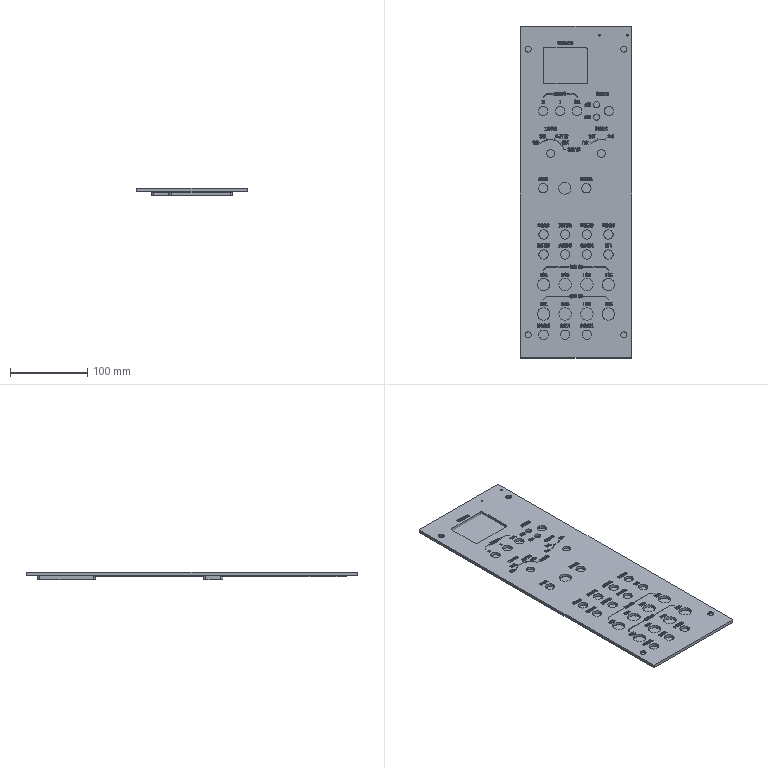NC program | Mastercam | posted with a generic post
Lines 8665 to 9754 of 54676:
(4 FEM |TOOL - 4|DIA. OFF. - 4|LEN. - 4|TOOL DIA. - 4.)
N7506 T4 M6
N7508 G0 G54 G90 X119.431 Y19.1 C0. B0. S7000 M3
N7510 G43 H4 Z50.
N7512 Z-4.248
N7514 G3 X119.931 Y18.6 I.5 F3000.
N7516 G1 X121.958
N7518 X121.975
N7520 G3 X122.265 Y18.641 J1.034
N7522 G1 X122.328 Y18.664
N7524 X122.449 Y18.722
N7526 X122.56 Y18.798
N7528 X122.659 Y18.889
N7530 X122.742 Y18.994
N7532 X122.81 Y19.11
N7534 X122.859 Y19.235
N7536 X122.888 Y19.366
N7538 G3 X122.9 Y19.529 I-1.149 J.163
N7540 G1 X122.899 Y19.539
N7542 X122.9 Y21.623
N7544 Y21.647 Z-4.249
N7546 Y21.71 Z-4.263
N7548 Y21.771 Z-4.303
N7550 Y21.808 Z-4.359
N7552 Y21.82 Z-4.423
N7554 Y21.808 Z-4.488
N7556 Y21.771 Z-4.544
N7558 Y21.71 Z-4.584
N7560 Y21.623 Z-4.599
N7562 Y19.539
N7564 Y19.531
N7566 G2 X122.876 Y19.3 I-1.123
N7568 G1 X122.859 Y19.235
N7570 X122.81 Y19.11
N7572 X122.742 Y18.994
N7574 X122.659 Y18.889
N7576 X122.56 Y18.798
N7578 X122.449 Y18.722
N7580 X122.328 Y18.664
N7582 X122.201 Y18.624
N7584 G2 X121.98 Y18.6 I-.221 J.986
N7586 G1 X121.958
N7588 X119.931
N7590 X119.907 Z-4.6
N7592 X119.845 Z-4.614
N7594 X119.783 Z-4.653
N7596 X119.746 Z-4.71
N7598 X119.734 Z-4.774
N7600 X119.746 Z-4.838
N7602 X119.783 Z-4.894
N7604 X119.845 Z-4.934
N7606 X119.931 Z-4.949
N7608 X121.958
N7610 X121.975
N7612 G3 X122.265 Y18.641 J1.034
N7614 G1 X122.328 Y18.664
N7616 X122.449 Y18.722
N7618 X122.56 Y18.798
N7620 X122.659 Y18.889
N7622 X122.742 Y18.994
N7624 X122.81 Y19.11
N7626 X122.859 Y19.235
N7628 X122.888 Y19.366
N7630 G3 X122.9 Y19.529 I-1.149 J.163
N7632 G1 X122.899 Y19.539
N7634 X122.9 Y21.623
N7636 Y21.647 Z-4.95
N7638 Y21.71 Z-4.964
N7640 Y21.771 Z-5.004
N7642 Y21.808 Z-5.06
N7644 Y21.82 Z-5.124
N7646 Y21.808 Z-5.188
N7648 Y21.771 Z-5.245
N7650 Y21.71 Z-5.284
N7652 Y21.623 Z-5.299
N7654 Y19.539
N7656 Y19.531
N7658 G2 X122.876 Y19.3 I-1.123
N7660 G1 X122.859 Y19.235
N7662 X122.81 Y19.11
N7664 X122.742 Y18.994
N7666 X122.659 Y18.889
N7668 X122.56 Y18.798
N7670 X122.449 Y18.722
N7672 X122.328 Y18.664
N7674 X122.201 Y18.624
N7676 G2 X121.98 Y18.6 I-.221 J.986
N7678 G1 X121.958
N7680 X119.931
N7682 X119.907 Z-5.3
N7684 X119.845 Z-5.314
N7686 X119.783 Z-5.354
N7688 X119.746 Z-5.41
N7690 X119.734 Z-5.474
N7692 X119.746 Z-5.539
N7694 X119.783 Z-5.595
N7696 X119.845 Z-5.635
N7698 X119.931 Z-5.65
N7700 X121.958
N7702 X121.975
N7704 G3 X122.265 Y18.641 J1.034
N7706 G1 X122.328 Y18.664
N7708 X122.449 Y18.722
N7710 X122.56 Y18.798
N7712 X122.659 Y18.889
N7714 X122.742 Y18.994
N7716 X122.81 Y19.11
N7718 X122.859 Y19.235
N7720 X122.888 Y19.366
N7722 G3 X122.9 Y19.529 I-1.149 J.163
N7724 G1 X122.899 Y19.539
N7726 X122.9 Y21.623
N7728 Y21.656 Z-5.652
N7730 Y21.709 Z-5.673
N7732 Y21.744 Z-5.708
N7734 Y21.764 Z-5.775
N7736 Y21.744 Z-5.842
N7738 Y21.709 Z-5.877
N7740 Y21.656 Z-5.897
N7742 Y21.623 Z-5.9
N7744 Y19.539
N7746 Y19.531
N7748 G2 X122.876 Y19.3 I-1.123
N7750 G1 X122.859 Y19.235
N7752 X122.81 Y19.11
N7754 X122.742 Y18.994
N7756 X122.659 Y18.889
N7758 X122.56 Y18.798
N7760 X122.449 Y18.722
N7762 X122.328 Y18.664
N7764 X122.201 Y18.624
N7766 G2 X121.98 Y18.6 I-.221 J.986
N7768 G1 X121.958
N7770 X119.931
N7772 X119.924 Z-5.897
N7774 Z-5.886
N7776 X119.931 Z-5.883
N7778 X121.958
N7780 X121.975
N7782 G3 X122.265 Y18.641 J1.034
N7784 G1 X122.328 Y18.664
N7786 X122.449 Y18.722
N7788 X122.56 Y18.798
N7790 X122.659 Y18.889
N7792 X122.742 Y18.994
N7794 X122.81 Y19.11
N7796 X122.859 Y19.235
N7798 X122.888 Y19.366
N7800 G3 X122.9 Y19.529 I-1.149 J.163
N7802 G1 X122.899 Y19.539
N7804 X122.9 Y21.623
N7806 G3 X122.4 Y22.123 I-.5
N7808 G0 Z50.
N7810 X119.395 Y8.9
N7812 Z-4.248
N7814 G2 X119.895 Y9.4 I.5
N7816 G1 X121.958
N7818 X121.975
N7820 G2 X122.265 Y9.359 J-1.034
N7822 G1 X122.389 Y9.31
N7824 X122.506 Y9.242
N7826 X122.611 Y9.159
N7828 X122.742 Y9.006
N7830 X122.81 Y8.889
N7832 X122.876 Y8.7
N7834 G2 X122.9 Y8.481 I-.981 J-.219
N7836 G1 Y8.46
N7838 Y6.328
N7840 Y6.304 Z-4.249
N7842 Y6.242 Z-4.263
N7844 Y6.18 Z-4.303
N7846 Y6.143 Z-4.359
N7848 Y6.131 Z-4.423
N7850 Y6.143 Z-4.488
N7852 Y6.18 Z-4.544
N7854 Y6.242 Z-4.584
N7856 Y6.328 Z-4.599
N7858 Y8.46
N7860 Y8.468
N7862 G3 X122.876 Y8.7 I-1.134
N7864 G1 X122.859 Y8.765
N7866 X122.81 Y8.889
N7868 X122.742 Y9.006
N7870 X122.611 Y9.159
N7872 X122.506 Y9.242
N7874 X122.389 Y9.31
N7876 X122.201 Y9.376
N7878 G3 X121.98 Y9.4 I-.221 J-.986
N7880 G1 X121.958
N7882 X119.895
N7884 X119.871 Z-4.6
N7886 X119.808 Z-4.614
N7888 X119.747 Z-4.653
N7890 X119.71 Z-4.71
N7892 X119.698 Z-4.774
N7894 X119.71 Z-4.838
N7896 X119.747 Z-4.894
N7898 X119.808 Z-4.934
N7900 X119.895 Z-4.949
N7902 X121.958
N7904 X121.975
N7906 G2 X122.265 Y9.359 J-1.034
N7908 G1 X122.389 Y9.31
N7910 X122.506 Y9.242
N7912 X122.611 Y9.159
N7914 X122.742 Y9.006
N7916 X122.81 Y8.889
N7918 X122.876 Y8.7
N7920 G2 X122.9 Y8.481 I-.981 J-.219
N7922 G1 Y8.46
N7924 Y6.328
N7926 Y6.304 Z-4.95
N7928 Y6.242 Z-4.964
N7930 Y6.18 Z-5.004
N7932 Y6.143 Z-5.06
N7934 Y6.131 Z-5.124
N7936 Y6.143 Z-5.188
N7938 Y6.18 Z-5.245
N7940 Y6.242 Z-5.284
N7942 Y6.328 Z-5.299
N7944 Y8.46
N7946 Y8.468
N7948 G3 X122.876 Y8.7 I-1.134
N7950 G1 X122.859 Y8.765
N7952 X122.81 Y8.889
N7954 X122.742 Y9.006
N7956 X122.611 Y9.159
N7958 X122.506 Y9.242
N7960 X122.389 Y9.31
N7962 X122.201 Y9.376
N7964 G3 X121.98 Y9.4 I-.221 J-.986
N7966 G1 X121.958
N7968 X119.895
N7970 X119.871 Z-5.3
N7972 X119.808 Z-5.314
N7974 X119.747 Z-5.354
N7976 X119.71 Z-5.41
N7978 X119.698 Z-5.474
N7980 X119.71 Z-5.539
N7982 X119.747 Z-5.595
N7984 X119.808 Z-5.635
N7986 X119.895 Z-5.65
N7988 X121.958
N7990 X121.975
N7992 G2 X122.265 Y9.359 J-1.034
N7994 G1 X122.389 Y9.31
N7996 X122.506 Y9.242
N7998 X122.611 Y9.159
N8000 X122.742 Y9.006
N8002 X122.81 Y8.889
N8004 X122.876 Y8.7
N8006 G2 X122.9 Y8.481 I-.981 J-.219
N8008 G1 Y8.46
N8010 Y6.328
N8012 Y6.295 Z-5.652
N8014 Y6.242 Z-5.673
N8016 Y6.207 Z-5.708
N8018 Y6.187 Z-5.775
N8020 Y6.207 Z-5.842
N8022 Y6.242 Z-5.877
N8024 Y6.295 Z-5.897
N8026 Y6.328 Z-5.9
N8028 Y8.46
N8030 Y8.468
N8032 G3 X122.876 Y8.7 I-1.134
N8034 G1 X122.859 Y8.765
N8036 X122.81 Y8.889
N8038 X122.742 Y9.006
N8040 X122.611 Y9.159
N8042 X122.506 Y9.242
N8044 X122.389 Y9.31
N8046 X122.201 Y9.376
N8048 G3 X121.98 Y9.4 I-.221 J-.986
N8050 G1 X121.958
N8052 X119.895
N8054 X119.888 Z-5.897
N8056 Z-5.886
N8058 X119.895 Z-5.884
N8060 X121.958
N8062 X121.975
N8064 G2 X122.265 Y9.359 J-1.034
N8066 G1 X122.389 Y9.31
N8068 X122.506 Y9.242
N8070 X122.611 Y9.159
N8072 X122.742 Y9.006
N8074 X122.81 Y8.889
N8076 X122.876 Y8.7
N8078 G2 X122.9 Y8.481 I-.981 J-.219
N8080 G1 Y8.46
N8082 Y6.328
N8084 G2 X122.4 Y5.828 I-.5
N8086 G0 Z50.
N8088 X90.674 Y8.9
N8090 Z-4.248
N8092 G3 X90.174 Y9.4 I-.5
N8094 G1 X88.04
N8096 X88.032
N8098 G3 X87.8 Y9.376 J-1.133
N8100 G1 X87.735 Y9.359
N8102 X87.61 Y9.31
N8104 X87.494 Y9.242
N8106 X87.389 Y9.159
N8108 X87.298 Y9.06
N8110 X87.222 Y8.949
N8112 X87.164 Y8.828
N8114 X87.124 Y8.7
N8116 G3 X87.1 Y8.481 I.979 J-.219
N8118 G1 Y8.46
N8120 Y6.292
N8122 Y6.268 Z-4.249
N8124 Y6.206 Z-4.263
N8126 Y6.144 Z-4.303
N8128 Y6.107 Z-4.359
N8130 Y6.095 Z-4.423
N8132 Y6.107 Z-4.488
N8134 Y6.144 Z-4.544
N8136 Y6.206 Z-4.584
N8138 Y6.292 Z-4.599
N8140 Y8.46
N8142 Y8.468
N8144 G2 X87.124 Y8.7 I1.135
N8146 G1 X87.141 Y8.765
N8148 X87.19 Y8.89
N8150 X87.258 Y9.006
N8152 X87.341 Y9.111
N8154 X87.44 Y9.202
N8156 X87.551 Y9.278
N8158 X87.672 Y9.336
N8160 X87.8 Y9.376
N8162 G2 X88.019 Y9.4 I.219 J-.978
N8164 G1 X88.04
N8166 X90.174
N8168 X90.198 Z-4.6
N8170 X90.261 Z-4.614
N8172 X90.322 Z-4.653
N8174 X90.359 Z-4.71
N8176 X90.371 Z-4.774
N8178 X90.359 Z-4.838
N8180 X90.322 Z-4.894
N8182 X90.261 Z-4.934
N8184 X90.174 Z-4.949
N8186 X88.04
N8188 X88.032
N8190 G3 X87.8 Y9.376 J-1.133
N8192 G1 X87.735 Y9.359
N8194 X87.61 Y9.31
N8196 X87.494 Y9.242
N8198 X87.389 Y9.159
N8200 X87.298 Y9.06
N8202 X87.222 Y8.949
N8204 X87.164 Y8.828
N8206 X87.124 Y8.7
N8208 G3 X87.1 Y8.481 I.979 J-.219
N8210 G1 Y8.46
N8212 Y6.292
N8214 Y6.268 Z-4.95
N8216 Y6.206 Z-4.964
N8218 Y6.144 Z-5.004
N8220 Y6.107 Z-5.06
N8222 Y6.095 Z-5.124
N8224 Y6.107 Z-5.188
N8226 Y6.144 Z-5.245
N8228 Y6.206 Z-5.284
N8230 Y6.292 Z-5.299
N8232 Y8.46
N8234 Y8.468
N8236 G2 X87.124 Y8.7 I1.135
N8238 G1 X87.141 Y8.765
N8240 X87.19 Y8.89
N8242 X87.258 Y9.006
N8244 X87.341 Y9.111
N8246 X87.44 Y9.202
N8248 X87.551 Y9.278
N8250 X87.672 Y9.336
N8252 X87.8 Y9.376
N8254 G2 X88.019 Y9.4 I.219 J-.978
N8256 G1 X88.04
N8258 X90.174
N8260 X90.198 Z-5.3
N8262 X90.261 Z-5.314
N8264 X90.322 Z-5.354
N8266 X90.359 Z-5.41
N8268 X90.371 Z-5.474
N8270 X90.359 Z-5.539
N8272 X90.322 Z-5.595
N8274 X90.261 Z-5.635
N8276 X90.174 Z-5.65
N8278 X88.04
N8280 X88.032
N8282 G3 X87.8 Y9.376 J-1.133
N8284 G1 X87.735 Y9.359
N8286 X87.61 Y9.31
N8288 X87.494 Y9.242
N8290 X87.389 Y9.159
N8292 X87.298 Y9.06
N8294 X87.222 Y8.949
N8296 X87.164 Y8.828
N8298 X87.124 Y8.7
N8300 G3 X87.1 Y8.481 I.979 J-.219
N8302 G1 Y8.46
N8304 Y6.292
N8306 Y6.259 Z-5.652
N8308 Y6.206 Z-5.673
N8310 Y6.171 Z-5.708
N8312 Y6.151 Z-5.775
N8314 Y6.171 Z-5.842
N8316 Y6.206 Z-5.877
N8318 Y6.259 Z-5.897
N8320 Y6.292 Z-5.9
N8322 Y8.46
N8324 Y8.468
N8326 G2 X87.124 Y8.7 I1.135
N8328 G1 X87.141 Y8.765
N8330 X87.19 Y8.89
N8332 X87.258 Y9.006
N8334 X87.341 Y9.111
N8336 X87.44 Y9.202
N8338 X87.551 Y9.278
N8340 X87.672 Y9.336
N8342 X87.8 Y9.376
N8344 G2 X88.019 Y9.4 I.219 J-.978
N8346 G1 X88.04
N8348 X90.174
N8350 X90.181 Z-5.897
N8352 Z-5.886
N8354 X90.174 Z-5.884
N8356 X88.04
N8358 X88.032
N8360 G3 X87.8 Y9.376 J-1.133
N8362 G1 X87.735 Y9.359
N8364 X87.61 Y9.31
N8366 X87.494 Y9.242
N8368 X87.389 Y9.159
N8370 X87.298 Y9.06
N8372 X87.222 Y8.949
N8374 X87.164 Y8.828
N8376 X87.124 Y8.7
N8378 G3 X87.1 Y8.481 I.979 J-.219
N8380 G1 Y8.46
N8382 Y6.292
N8384 G3 X87.6 Y5.792 I.5
N8386 G0 Z50.
N8388 X90.711 Y19.1
N8390 Z-4.248
N8392 G2 X90.211 Y18.6 I-.5
N8394 G1 X88.04
N8396 X88.025
N8398 G2 X87.735 Y18.641 J1.036
N8400 G1 X87.672 Y18.664
N8402 X87.551 Y18.722
N8404 X87.389 Y18.841
N8406 X87.298 Y18.94
N8408 X87.222 Y19.051
N8410 X87.163 Y19.172
N8412 X87.124 Y19.3
N8414 X87.104 Y19.433
N8416 X87.1 Y21.587
N8418 Y21.611 Z-4.249
N8420 Y21.673 Z-4.263
N8422 Y21.735 Z-4.303
N8424 Y21.772 Z-4.359
N8426 Y21.784 Z-4.423
N8428 Y21.772 Z-4.488
N8430 Y21.735 Z-4.544
N8432 Y21.673 Z-4.584
N8434 Y21.587 Z-4.599
N8436 Y19.539
N8438 Y19.531
N8440 G3 X87.124 Y19.3 I1.123
N8442 G1 X87.141 Y19.235
N8444 X87.191 Y19.11
N8446 X87.258 Y18.994
N8448 X87.341 Y18.889
N8450 X87.439 Y18.798
N8452 X87.551 Y18.722
N8454 X87.672 Y18.664
N8456 X87.735 Y18.641
N8458 X87.865 Y18.612
N8460 G3 X88.031 Y18.6 I.166 J1.164
N8462 G1 X88.04
N8464 X90.211
N8466 X90.234 Z-4.6
N8468 X90.297 Z-4.614
N8470 X90.358 Z-4.653
N8472 X90.395 Z-4.71
N8474 X90.408 Z-4.774
N8476 X90.395 Z-4.838
N8478 X90.358 Z-4.894
N8480 X90.297 Z-4.934
N8482 X90.211 Z-4.949
N8484 X88.04
N8486 X88.025
N8488 G2 X87.735 Y18.641 J1.036
N8490 G1 X87.672 Y18.664
N8492 X87.551 Y18.722
N8494 X87.389 Y18.841
N8496 X87.298 Y18.94
N8498 X87.222 Y19.051
N8500 X87.163 Y19.172
N8502 X87.124 Y19.3
N8504 X87.104 Y19.433
N8506 X87.1 Y21.587
N8508 Y21.611 Z-4.95
N8510 Y21.673 Z-4.964
N8512 Y21.735 Z-5.004
N8514 Y21.772 Z-5.06
N8516 Y21.784 Z-5.124
N8518 Y21.772 Z-5.188
N8520 Y21.735 Z-5.245
N8522 Y21.673 Z-5.284
N8524 Y21.587 Z-5.299
N8526 Y19.539
N8528 Y19.531
N8530 G3 X87.124 Y19.3 I1.123
N8532 G1 X87.141 Y19.235
N8534 X87.191 Y19.11
N8536 X87.258 Y18.994
N8538 X87.341 Y18.889
N8540 X87.439 Y18.798
N8542 X87.551 Y18.722
N8544 X87.672 Y18.664
N8546 X87.735 Y18.641
N8548 X87.865 Y18.612
N8550 G3 X88.031 Y18.6 I.166 J1.164
N8552 G1 X88.04
N8554 X90.211
N8556 X90.234 Z-5.3
N8558 X90.297 Z-5.314
N8560 X90.358 Z-5.354
N8562 X90.395 Z-5.41
N8564 X90.408 Z-5.474
N8566 X90.395 Z-5.539
N8568 X90.358 Z-5.595
N8570 X90.297 Z-5.635
N8572 X90.211 Z-5.65
N8574 X88.04
N8576 X88.025
N8578 G2 X87.735 Y18.641 J1.036
N8580 G1 X87.672 Y18.664
N8582 X87.551 Y18.722
N8584 X87.389 Y18.841
N8586 X87.298 Y18.94
N8588 X87.222 Y19.051
N8590 X87.163 Y19.172
N8592 X87.124 Y19.3
N8594 X87.104 Y19.433
N8596 X87.1 Y21.587
N8598 Y21.62 Z-5.652
N8600 Y21.673 Z-5.673
N8602 Y21.708 Z-5.708
N8604 Y21.728 Z-5.775
N8606 Y21.708 Z-5.842
N8608 Y21.673 Z-5.877
N8610 Y21.62 Z-5.897
N8612 Y21.587 Z-5.9
N8614 Y19.539
N8616 Y19.531
N8618 G3 X87.124 Y19.3 I1.123
N8620 G1 X87.141 Y19.235
N8622 X87.191 Y19.11
N8624 X87.258 Y18.994
N8626 X87.341 Y18.889
N8628 X87.439 Y18.798
N8630 X87.551 Y18.722
N8632 X87.672 Y18.664
N8634 X87.735 Y18.641
N8636 X87.865 Y18.612
N8638 G3 X88.031 Y18.6 I.166 J1.164
N8640 G1 X88.04
N8642 X90.211
N8644 X90.218 Z-5.897
N8646 Z-5.886
N8648 X90.211 Z-5.883
N8650 X88.04
N8652 X88.025
N8654 G2 X87.735 Y18.641 J1.036
N8656 G1 X87.672 Y18.664
N8658 X87.551 Y18.722
N8660 X87.389 Y18.841
N8662 X87.298 Y18.94
N8664 X87.222 Y19.051
N8666 X87.163 Y19.172
N8668 X87.124 Y19.3
N8670 X87.104 Y19.433
N8672 X87.1 Y21.587
N8674 G2 X87.6 Y22.087 I.5
N8676 G0 Z50.
N8678 X22.4 Y27.813
N8680 Z-4.248
N8682 G3 X22.9 Y28.313 J.5
N8684 G1 Y30.461
N8686 Y30.469
N8688 G3 X22.876 Y30.7 I-1.123
N8690 G1 X22.859 Y30.765
N8692 X22.81 Y30.89
N8694 X22.742 Y31.006
N8696 X22.659 Y31.111
N8698 X22.56 Y31.202
N8700 X22.449 Y31.278
N8702 X22.328 Y31.336
N8704 X22.2 Y31.376
N8706 X22.067 Y31.396
N8708 X19.838 Y31.4
N8710 X19.814 Z-4.249
N8712 X19.751 Z-4.263
N8714 X19.69 Z-4.303
N8716 X19.653 Z-4.359
N8718 X19.641 Z-4.423
N8720 X19.653 Z-4.488
N8722 X19.69 Z-4.544
N8724 X19.751 Z-4.584
N8726 X19.838 Z-4.599
N8728 X21.961
N8730 X21.969
N8732 G2 X22.2 Y31.376 J-1.123
N8734 G1 X22.265 Y31.359
N8736 X22.39 Y31.31
N8738 X22.506 Y31.242
N8740 X22.611 Y31.159
N8742 X22.702 Y31.06
N8744 X22.778 Y30.949
N8746 X22.836 Y30.828
N8748 X22.876 Y30.7
N8750 X22.896 Y30.567
N8752 X22.9 Y28.313
N8754 Y28.289 Z-4.6
N8756 Y28.227 Z-4.614
N8758 Y28.165 Z-4.653
N8760 Y28.128 Z-4.71
N8762 Y28.116 Z-4.774
N8764 Y28.128 Z-4.838
N8766 Y28.165 Z-4.894
N8768 Y28.227 Z-4.934
N8770 Y28.313 Z-4.949
N8772 Y30.461
N8774 Y30.469
N8776 G3 X22.876 Y30.7 I-1.123
N8778 G1 X22.859 Y30.765
N8780 X22.81 Y30.89
N8782 X22.742 Y31.006
N8784 X22.659 Y31.111
N8786 X22.56 Y31.202
N8788 X22.449 Y31.278
N8790 X22.328 Y31.336
N8792 X22.2 Y31.376
N8794 X22.067 Y31.396
N8796 X19.838 Y31.4
N8798 X19.814 Z-4.95
N8800 X19.751 Z-4.964
N8802 X19.69 Z-5.004
N8804 X19.653 Z-5.06
N8806 X19.641 Z-5.124
N8808 X19.653 Z-5.188
N8810 X19.69 Z-5.245
N8812 X19.751 Z-5.284
N8814 X19.838 Z-5.299
N8816 X21.961
N8818 X21.969
N8820 G2 X22.2 Y31.376 J-1.123
N8822 G1 X22.265 Y31.359
N8824 X22.39 Y31.31
N8826 X22.506 Y31.242
N8828 X22.611 Y31.159
N8830 X22.702 Y31.06
N8832 X22.778 Y30.949
N8834 X22.836 Y30.828
N8836 X22.876 Y30.7
N8838 X22.896 Y30.567
N8840 X22.9 Y28.313
N8842 Y28.289 Z-5.3
N8844 Y28.227 Z-5.314
N8846 Y28.165 Z-5.354
N8848 Y28.128 Z-5.41
N8850 Y28.116 Z-5.474
N8852 Y28.128 Z-5.539
N8854 Y28.165 Z-5.595
N8856 Y28.227 Z-5.635
N8858 Y28.313 Z-5.65
N8860 Y30.461
N8862 Y30.469
N8864 G3 X22.876 Y30.7 I-1.123
N8866 G1 X22.859 Y30.765
N8868 X22.81 Y30.89
N8870 X22.742 Y31.006
N8872 X22.659 Y31.111
N8874 X22.56 Y31.202
N8876 X22.449 Y31.278
N8878 X22.328 Y31.336
N8880 X22.2 Y31.376
N8882 X22.067 Y31.396
N8884 X19.838 Y31.4
N8886 X19.805 Z-5.652
N8888 X19.752 Z-5.673
N8890 X19.717 Z-5.708
N8892 X19.697 Z-5.775
N8894 X19.717 Z-5.842
N8896 X19.752 Z-5.877
N8898 X19.805 Z-5.897
N8900 X19.838 Z-5.9
N8902 X21.961
N8904 X21.969
N8906 G2 X22.2 Y31.376 J-1.123
N8908 G1 X22.265 Y31.359
N8910 X22.39 Y31.31
N8912 X22.506 Y31.242
N8914 X22.611 Y31.159
N8916 X22.702 Y31.06
N8918 X22.778 Y30.949
N8920 X22.836 Y30.828
N8922 X22.876 Y30.7
N8924 X22.896 Y30.567
N8926 X22.9 Y28.313
N8928 Y28.306 Z-5.897
N8930 Z-5.886
N8932 Y28.313 Z-5.883
N8934 Y30.461
N8936 Y30.469
N8938 G3 X22.876 Y30.7 I-1.123
N8940 G1 X22.859 Y30.765
N8942 X22.81 Y30.89
N8944 X22.742 Y31.006
N8946 X22.659 Y31.111
N8948 X22.56 Y31.202
N8950 X22.449 Y31.278
N8952 X22.328 Y31.336
N8954 X22.2 Y31.376
N8956 X22.067 Y31.396
N8958 X19.838 Y31.4
N8960 G3 X19.338 Y30.9 J-.5
N8962 G0 Z50.
N8964 X-9.383
N8966 Z-4.248
N8968 G3 X-9.883 Y31.4 I-.5
N8970 G1 X-11.961
N8972 X-11.976
N8974 G3 X-12.263 Y31.359 J-1.028
N8976 G1 X-12.329 Y31.336
N8978 X-12.449 Y31.278
N8980 X-12.56 Y31.202
N8982 G3 X-12.742 Y31.007 I.655 J-.79
N8984 G1 X-12.779 Y30.948
N8986 X-12.859 Y30.765
N8988 X-12.888 Y30.634
N8990 G3 X-12.9 Y30.471 I1.149 J-.163
N8992 G1 X-12.899 Y30.461
N8994 X-12.9 Y28.277
N8996 Y28.253 Z-4.249
N8998 Y28.19 Z-4.263
N9000 Y28.129 Z-4.303
N9002 Y28.092 Z-4.359
N9004 Y28.08 Z-4.423
N9006 Y28.092 Z-4.488
N9008 Y28.129 Z-4.544
N9010 Y28.19 Z-4.584
N9012 Y28.277 Z-4.599
N9014 Y30.461
N9016 Y30.469
N9018 G2 X-12.876 Y30.7 I1.123
N9020 G1 X-12.859 Y30.765
N9022 X-12.779 Y30.948
N9024 X-12.702 Y31.06
N9026 G2 X-12.506 Y31.242 I.784 J-.649
N9028 G1 X-12.449 Y31.278
N9030 X-12.329 Y31.336
N9032 X-12.263 Y31.359
N9034 X-12.067 Y31.396
N9036 X-9.883 Y31.4
N9038 X-9.859 Z-4.6
N9040 X-9.796 Z-4.614
N9042 X-9.735 Z-4.653
N9044 X-9.698 Z-4.71
N9046 X-9.686 Z-4.774
N9048 X-9.698 Z-4.838
N9050 X-9.735 Z-4.894
N9052 X-9.796 Z-4.934
N9054 X-9.883 Z-4.949
N9056 X-11.961
N9058 X-11.976
N9060 G3 X-12.263 Y31.359 J-1.028
N9062 G1 X-12.329 Y31.336
N9064 X-12.449 Y31.278
N9066 X-12.56 Y31.202
N9068 G3 X-12.742 Y31.007 I.655 J-.79
N9070 G1 X-12.779 Y30.948
N9072 X-12.859 Y30.765
N9074 X-12.888 Y30.634
N9076 G3 X-12.9 Y30.471 I1.149 J-.163
N9078 G1 X-12.899 Y30.461
N9080 X-12.9 Y28.277
N9082 Y28.253 Z-4.95
N9084 Y28.19 Z-4.964
N9086 Y28.129 Z-5.004
N9088 Y28.092 Z-5.06
N9090 Y28.08 Z-5.124
N9092 Y28.092 Z-5.188
N9094 Y28.129 Z-5.245
N9096 Y28.19 Z-5.284
N9098 Y28.277 Z-5.299
N9100 Y30.461
N9102 Y30.469
N9104 G2 X-12.876 Y30.7 I1.123
N9106 G1 X-12.859 Y30.765
N9108 X-12.779 Y30.948
N9110 X-12.702 Y31.06
N9112 G2 X-12.506 Y31.242 I.784 J-.649
N9114 G1 X-12.449 Y31.278
N9116 X-12.329 Y31.336
N9118 X-12.263 Y31.359
N9120 X-12.067 Y31.396
N9122 X-9.883 Y31.4
N9124 X-9.859 Z-5.3
N9126 X-9.796 Z-5.314
N9128 X-9.735 Z-5.354
N9130 X-9.698 Z-5.41
N9132 X-9.686 Z-5.474
N9134 X-9.698 Z-5.539
N9136 X-9.735 Z-5.595
N9138 X-9.796 Z-5.635
N9140 X-9.883 Z-5.65
N9142 X-11.961
N9144 X-11.976
N9146 G3 X-12.263 Y31.359 J-1.028
N9148 G1 X-12.329 Y31.336
N9150 X-12.449 Y31.278
N9152 X-12.56 Y31.202
N9154 G3 X-12.742 Y31.007 I.655 J-.79
N9156 G1 X-12.779 Y30.948
N9158 X-12.859 Y30.765
N9160 X-12.888 Y30.634
N9162 G3 X-12.9 Y30.471 I1.149 J-.163
N9164 G1 X-12.899 Y30.461
N9166 X-12.9 Y28.277
N9168 Y28.244 Z-5.652
N9170 Y28.191 Z-5.673
N9172 Y28.156 Z-5.708
N9174 Y28.136 Z-5.775
N9176 Y28.156 Z-5.842
N9178 Y28.191 Z-5.877
N9180 Y28.244 Z-5.897
N9182 Y28.277 Z-5.9
N9184 Y30.461
N9186 Y30.469
N9188 G2 X-12.876 Y30.7 I1.123
N9190 G1 X-12.859 Y30.765
N9192 X-12.779 Y30.948
N9194 X-12.702 Y31.06
N9196 G2 X-12.506 Y31.242 I.784 J-.649
N9198 G1 X-12.449 Y31.278
N9200 X-12.329 Y31.336
N9202 X-12.263 Y31.359
N9204 X-12.067 Y31.396
N9206 X-9.883 Y31.4
N9208 X-9.876 Z-5.897
N9210 Z-5.886
N9212 X-9.883 Z-5.883
N9214 X-11.961
N9216 X-11.976
N9218 G3 X-12.263 Y31.359 J-1.028
N9220 G1 X-12.329 Y31.336
N9222 X-12.449 Y31.278
N9224 X-12.56 Y31.202
N9226 G3 X-12.742 Y31.007 I.655 J-.79
N9228 G1 X-12.779 Y30.948
N9230 X-12.859 Y30.765
N9232 X-12.888 Y30.634
N9234 G3 X-12.9 Y30.471 I1.149 J-.163
N9236 G1 X-12.899 Y30.461
N9238 X-12.9 Y28.277
N9240 G3 X-12.4 Y27.777 I.5
N9242 G0 Z50.
N9244 X-42.6 Y20.292
N9246 Z-4.248
N9248 G3 X-42.1 Y20.792 J.5
N9250 G1 Y22.96
N9252 Y22.978
N9254 G3 X-42.141 Y23.265 I-1.014
N9256 G1 X-42.164 Y23.328
N9258 X-42.257 Y23.505
N9260 X-42.342 Y23.612
N9262 X-42.494 Y23.742
N9264 X-42.61 Y23.81
N9266 X-42.735 Y23.859
N9268 X-42.866 Y23.888
N9270 G3 X-43.03 Y23.9 I-.164 J-1.16
N9272 G1 X-43.042
N9274 X-45.178
N9276 X-45.202 Z-4.249
N9278 X-45.264 Z-4.263
N9280 X-45.325 Z-4.303
N9282 X-45.362 Z-4.359
N9284 X-45.375 Z-4.423
N9286 X-45.362 Z-4.488
N9288 X-45.325 Z-4.544
N9290 X-45.264 Z-4.584
N9292 X-45.178 Z-4.599
N9294 X-43.042
N9296 X-43.024
N9298 G2 X-42.735 Y23.859 J-1.026
N9300 G1 X-42.672 Y23.836
N9302 X-42.551 Y23.778
N9304 X-42.44 Y23.703
N9306 X-42.342 Y23.612
N9308 X-42.257 Y23.505
N9310 X-42.164 Y23.328
N9312 X-42.141 Y23.265
N9314 X-42.112 Y23.133
N9316 G2 X-42.1 Y22.969 I-1.161 J-.164
N9318 G1 X-42.101 Y22.96
N9320 X-42.1 Y20.792
N9322 Y20.768 Z-4.6
N9324 Y20.705 Z-4.614
N9326 Y20.644 Z-4.653
N9328 Y20.607 Z-4.71
N9330 Y20.595 Z-4.774
N9332 Y20.607 Z-4.838
N9334 Y20.644 Z-4.894
N9336 Y20.705 Z-4.934
N9338 Y20.792 Z-4.949
N9340 Y22.96
N9342 Y22.978
N9344 G3 X-42.141 Y23.265 I-1.014
N9346 G1 X-42.164 Y23.328
N9348 X-42.257 Y23.505
N9350 X-42.342 Y23.612
N9352 X-42.494 Y23.742
N9354 X-42.61 Y23.81
N9356 X-42.735 Y23.859
N9358 X-42.866 Y23.888
N9360 G3 X-43.03 Y23.9 I-.164 J-1.16
N9362 G1 X-43.042
N9364 X-45.178
N9366 X-45.202 Z-4.95
N9368 X-45.264 Z-4.964
N9370 X-45.325 Z-5.004
N9372 X-45.362 Z-5.06
N9374 X-45.375 Z-5.124
N9376 X-45.362 Z-5.188
N9378 X-45.325 Z-5.245
N9380 X-45.264 Z-5.284
N9382 X-45.178 Z-5.299
N9384 X-43.042
N9386 X-43.024
N9388 G2 X-42.735 Y23.859 J-1.026
N9390 G1 X-42.672 Y23.836
N9392 X-42.551 Y23.778
N9394 X-42.44 Y23.703
N9396 X-42.342 Y23.612
N9398 X-42.257 Y23.505
N9400 X-42.164 Y23.328
N9402 X-42.141 Y23.265
N9404 X-42.112 Y23.133
N9406 G2 X-42.1 Y22.969 I-1.161 J-.164
N9408 G1 X-42.101 Y22.96
N9410 X-42.1 Y20.792
N9412 Y20.768 Z-5.3
N9414 Y20.705 Z-5.314
N9416 Y20.644 Z-5.354
N9418 Y20.607 Z-5.41
N9420 Y20.595 Z-5.474
N9422 Y20.607 Z-5.539
N9424 Y20.644 Z-5.595
N9426 Y20.705 Z-5.635
N9428 Y20.792 Z-5.65
N9430 Y22.96
N9432 Y22.978
N9434 G3 X-42.141 Y23.265 I-1.014
N9436 G1 X-42.164 Y23.328
N9438 X-42.257 Y23.505
N9440 X-42.342 Y23.612
N9442 X-42.494 Y23.742
N9444 X-42.61 Y23.81
N9446 X-42.735 Y23.859
N9448 X-42.866 Y23.888
N9450 G3 X-43.03 Y23.9 I-.164 J-1.16
N9452 G1 X-43.042
N9454 X-45.178
N9456 X-45.211 Z-5.652
N9458 X-45.264 Z-5.673
N9460 X-45.299 Z-5.708
N9462 X-45.319 Z-5.775
N9464 X-45.299 Z-5.842
N9466 X-45.264 Z-5.877
N9468 X-45.211 Z-5.897
N9470 X-45.178 Z-5.9
N9472 X-43.042
N9474 X-43.024
N9476 G2 X-42.735 Y23.859 J-1.026
N9478 G1 X-42.672 Y23.836
N9480 X-42.551 Y23.778
N9482 X-42.44 Y23.703
N9484 X-42.342 Y23.612
N9486 X-42.257 Y23.505
N9488 X-42.164 Y23.328
N9490 X-42.141 Y23.265
N9492 X-42.112 Y23.133
N9494 G2 X-42.1 Y22.969 I-1.161 J-.164
N9496 G1 X-42.101 Y22.96
N9498 X-42.1 Y20.792
N9500 Y20.785 Z-5.897
N9502 Z-5.886
N9504 Y20.792 Z-5.884
N9506 Y22.96
N9508 Y22.978
N9510 G3 X-42.141 Y23.265 I-1.014
N9512 G1 X-42.164 Y23.328
N9514 X-42.257 Y23.505
N9516 X-42.342 Y23.612
N9518 X-42.494 Y23.742
N9520 X-42.61 Y23.81
N9522 X-42.735 Y23.859
N9524 X-42.866 Y23.888
N9526 G3 X-43.03 Y23.9 I-.164 J-1.16
N9528 G1 X-43.042
N9530 X-45.178
N9532 G3 X-45.678 Y23.4 J-.5
N9534 G0 Z50.
N9536 X-45.642 Y32.6
N9538 Z-4.248
N9540 G3 X-45.142 Y32.1 I.5
N9542 G1 X-43.042
N9544 X-43.025
N9546 G3 X-42.736 Y32.141 J1.033
N9548 G1 X-42.61 Y32.19
N9550 X-42.494 Y32.258
N9552 X-42.389 Y32.341
N9554 X-42.298 Y32.44
N9556 X-42.222 Y32.551
N9558 X-42.164 Y32.672
N9560 X-42.124 Y32.8
N9562 X-42.104 Y32.933
N9564 X-42.1 Y35.219
N9566 Y35.243 Z-4.249
N9568 Y35.305 Z-4.263
N9570 Y35.367 Z-4.303
N9572 Y35.404 Z-4.359
N9574 Y35.416 Z-4.423
N9576 Y35.404 Z-4.488
N9578 Y35.367 Z-4.544
N9580 Y35.305 Z-4.584
N9582 Y35.219 Z-4.599
N9584 Y33.039
N9586 Y33.031
N9588 G2 X-42.124 Y32.8 I-1.123
N9590 G1 X-42.141 Y32.735
N9592 X-42.19 Y32.61
N9594 X-42.258 Y32.494
N9596 X-42.341 Y32.389
N9598 X-42.44 Y32.298
N9600 X-42.551 Y32.222
N9602 X-42.61 Y32.19
N9604 X-42.736 Y32.141
N9606 X-42.932 Y32.104
N9608 X-45.142 Y32.1
N9610 X-45.165 Z-4.6
N9612 X-45.228 Z-4.614
N9614 X-45.289 Z-4.653
N9616 X-45.326 Z-4.71
N9618 X-45.339 Z-4.774
N9620 X-45.326 Z-4.838
N9622 X-45.289 Z-4.894
N9624 X-45.228 Z-4.934
N9626 X-45.142 Z-4.949
N9628 X-43.042
N9630 X-43.025
N9632 G3 X-42.736 Y32.141 J1.033
N9634 G1 X-42.61 Y32.19
N9636 X-42.494 Y32.258
N9638 X-42.389 Y32.341
N9640 X-42.298 Y32.44
N9642 X-42.222 Y32.551
N9644 X-42.164 Y32.672
N9646 X-42.124 Y32.8
N9648 X-42.104 Y32.933
N9650 X-42.1 Y35.219
N9652 Y35.243 Z-4.95
N9654 Y35.305 Z-4.964
N9656 Y35.367 Z-5.004
N9658 Y35.404 Z-5.06
N9660 Y35.416 Z-5.124
N9662 Y35.404 Z-5.188
N9664 Y35.367 Z-5.245
N9666 Y35.305 Z-5.284
N9668 Y35.219 Z-5.299
N9670 Y33.039
N9672 Y33.031
N9674 G2 X-42.124 Y32.8 I-1.123
N9676 G1 X-42.141 Y32.735
N9678 X-42.19 Y32.61
N9680 X-42.258 Y32.494
N9682 X-42.341 Y32.389